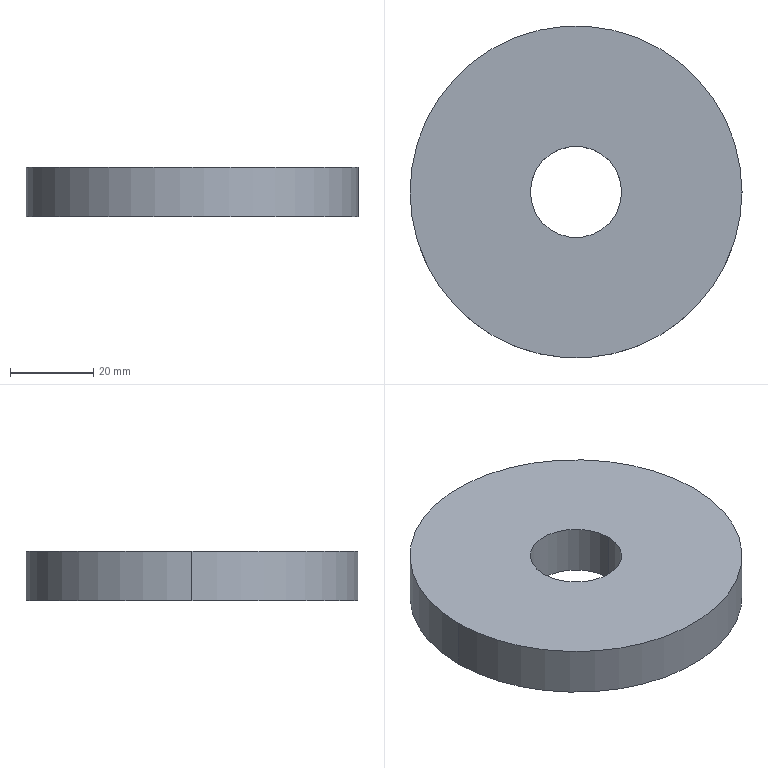Part | SolidWorks | features Extrusion 1 | 1 solid | 6 faces | box 80 x 80 x 12 mm | volume 55757 mm3 | cylinder 4 | plane 2 | commonest cylinder face diameters 22 x2 80 x2
STEP:
#1=CARTESIAN_POINT('',(-11.,0.,12.));
#2=VERTEX_POINT('',#1);
#3=CARTESIAN_POINT('',(11.,0.,12.));
#4=VERTEX_POINT('',#3);
#5=CARTESIAN_POINT('',(0.,0.,12.));
#6=DIRECTION('',(0.,0.,1.));
#7=DIRECTION('',(1.,0.,0.));
#8=AXIS2_PLACEMENT_3D('',#5,#6,#7);
#9=CIRCLE('',#8,11.);
#10=EDGE_CURVE('',#2,#4,#9,.T.);
#11=ORIENTED_EDGE('',*,*,#10,.T.);
#12=CARTESIAN_POINT('',(11.,0.,0.));
#13=VERTEX_POINT('',#12);
#14=CARTESIAN_POINT('',(11.,0.,12.));
#15=DIRECTION('',(0.,0.,-1.));
#16=VECTOR('',#15,1000.);
#17=LINE('',#14,#16);
#18=EDGE_CURVE('',#4,#13,#17,.T.);
#19=ORIENTED_EDGE('',*,*,#18,.T.);
#20=CARTESIAN_POINT('',(-11.,0.,0.));
#21=VERTEX_POINT('',#20);
#22=CARTESIAN_POINT('',(0.,0.,0.));
#23=DIRECTION('',(0.,0.,1.));
#24=DIRECTION('',(1.,0.,0.));
#25=AXIS2_PLACEMENT_3D('',#22,#23,#24);
#26=CIRCLE('',#25,11.);
#27=EDGE_CURVE('',#21,#13,#26,.T.);
#28=ORIENTED_EDGE('',*,*,#27,.F.);
#29=CARTESIAN_POINT('',(-11.,0.,12.));
#30=DIRECTION('',(0.,0.,-1.));
#31=VECTOR('',#30,1000.);
#32=LINE('',#29,#31);
#33=EDGE_CURVE('',#2,#21,#32,.T.);
#34=ORIENTED_EDGE('',*,*,#33,.F.);
#35=EDGE_LOOP('',(#11,#19,#28,#34));
#36=FACE_OUTER_BOUND('',#35,.T.);
#37=CARTESIAN_POINT('',(0.,0.,12.));
#38=DIRECTION('',(0.,0.,-1.));
#39=DIRECTION('',(-1.,0.,0.));
#40=AXIS2_PLACEMENT_3D('',#37,#38,#39);
#41=CYLINDRICAL_SURFACE('',#40,11.);
#42=ADVANCED_FACE('',(#36),#41,.F.);
#43=CARTESIAN_POINT('',(40.,0.,12.));
#44=VERTEX_POINT('',#43);
#45=CARTESIAN_POINT('',(-40.,0.,12.));
#46=VERTEX_POINT('',#45);
#47=CARTESIAN_POINT('',(0.,0.,12.));
#48=DIRECTION('',(0.,0.,1.));
#49=DIRECTION('',(1.,0.,0.));
#50=AXIS2_PLACEMENT_3D('',#47,#48,#49);
#51=CIRCLE('',#50,40.);
#52=EDGE_CURVE('',#44,#46,#51,.T.);
#53=ORIENTED_EDGE('',*,*,#52,.F.);
#54=CARTESIAN_POINT('',(40.,0.,0.));
#55=VERTEX_POINT('',#54);
#56=CARTESIAN_POINT('',(40.,0.,12.));
#57=DIRECTION('',(0.,0.,-1.));
#58=VECTOR('',#57,1000.);
#59=LINE('',#56,#58);
#60=EDGE_CURVE('',#44,#55,#59,.T.);
#61=ORIENTED_EDGE('',*,*,#60,.T.);
#62=CARTESIAN_POINT('',(-40.,0.,0.));
#63=VERTEX_POINT('',#62);
#64=CARTESIAN_POINT('',(0.,0.,0.));
#65=DIRECTION('',(0.,0.,1.));
#66=DIRECTION('',(1.,0.,0.));
#67=AXIS2_PLACEMENT_3D('',#64,#65,#66);
#68=CIRCLE('',#67,40.);
#69=EDGE_CURVE('',#55,#63,#68,.T.);
#70=ORIENTED_EDGE('',*,*,#69,.T.);
#71=CARTESIAN_POINT('',(-40.,0.,12.));
#72=DIRECTION('',(0.,0.,-1.));
#73=VECTOR('',#72,1000.);
#74=LINE('',#71,#73);
#75=EDGE_CURVE('',#46,#63,#74,.T.);
#76=ORIENTED_EDGE('',*,*,#75,.F.);
#77=EDGE_LOOP('',(#53,#61,#70,#76));
#78=FACE_OUTER_BOUND('',#77,.T.);
#79=CARTESIAN_POINT('',(0.,0.,12.));
#80=DIRECTION('',(0.,0.,-1.));
#81=DIRECTION('',(-1.,0.,0.));
#82=AXIS2_PLACEMENT_3D('',#79,#80,#81);
#83=CYLINDRICAL_SURFACE('',#82,40.);
#84=ADVANCED_FACE('',(#78),#83,.T.);
#85=CARTESIAN_POINT('',(0.,0.,12.));
#86=DIRECTION('',(0.,0.,1.));
#87=DIRECTION('',(1.,0.,0.));
#88=AXIS2_PLACEMENT_3D('',#85,#86,#87);
#89=CIRCLE('',#88,40.);
#90=EDGE_CURVE('',#46,#44,#89,.T.);
#91=ORIENTED_EDGE('',*,*,#90,.T.);
#92=ORIENTED_EDGE('',*,*,#52,.T.);
#93=EDGE_LOOP('',(#91,#92));
#94=FACE_OUTER_BOUND('',#93,.T.);
#95=ORIENTED_EDGE('',*,*,#10,.F.);
#96=CARTESIAN_POINT('',(0.,0.,12.));
#97=DIRECTION('',(0.,0.,1.));
#98=DIRECTION('',(1.,0.,0.));
#99=AXIS2_PLACEMENT_3D('',#96,#97,#98);
#100=CIRCLE('',#99,11.);
#101=EDGE_CURVE('',#4,#2,#100,.T.);
#102=ORIENTED_EDGE('',*,*,#101,.F.);
#103=EDGE_LOOP('',(#95,#102));
#104=FACE_BOUND('',#103,.T.);
#105=CARTESIAN_POINT('',(0.,0.,12.));
#106=DIRECTION('',(0.,0.,1.));
#107=DIRECTION('',(1.,0.,0.));
#108=AXIS2_PLACEMENT_3D('',#105,#106,#107);
#109=PLANE('',#108);
#110=ADVANCED_FACE('',(#94,#104),#109,.T.);
#111=CARTESIAN_POINT('',(0.,0.,0.));
#112=DIRECTION('',(0.,0.,1.));
#113=DIRECTION('',(1.,0.,0.));
#114=AXIS2_PLACEMENT_3D('',#111,#112,#113);
#115=CIRCLE('',#114,40.);
#116=EDGE_CURVE('',#63,#55,#115,.T.);
#117=ORIENTED_EDGE('',*,*,#116,.F.);
#118=ORIENTED_EDGE('',*,*,#69,.F.);
#119=EDGE_LOOP('',(#117,#118));
#120=FACE_OUTER_BOUND('',#119,.T.);
#121=ORIENTED_EDGE('',*,*,#27,.T.);
#122=CARTESIAN_POINT('',(0.,0.,0.));
#123=DIRECTION('',(0.,0.,1.));
#124=DIRECTION('',(1.,0.,0.));
#125=AXIS2_PLACEMENT_3D('',#122,#123,#124);
#126=CIRCLE('',#125,11.);
#127=EDGE_CURVE('',#13,#21,#126,.T.);
#128=ORIENTED_EDGE('',*,*,#127,.T.);
#129=EDGE_LOOP('',(#121,#128));
#130=FACE_BOUND('',#129,.T.);
#131=CARTESIAN_POINT('',(0.,0.,0.));
#132=DIRECTION('',(0.,0.,1.));
#133=DIRECTION('',(1.,0.,0.));
#134=AXIS2_PLACEMENT_3D('',#131,#132,#133);
#135=PLANE('',#134);
#136=ADVANCED_FACE('',(#120,#130),#135,.F.);
#137=ORIENTED_EDGE('',*,*,#60,.F.);
#138=ORIENTED_EDGE('',*,*,#90,.F.);
#139=ORIENTED_EDGE('',*,*,#75,.T.);
#140=ORIENTED_EDGE('',*,*,#116,.T.);
#141=EDGE_LOOP('',(#137,#138,#139,#140));
#142=FACE_OUTER_BOUND('',#141,.T.);
#143=CARTESIAN_POINT('',(0.,0.,12.));
#144=DIRECTION('',(0.,0.,-1.));
#145=DIRECTION('',(-1.,0.,0.));
#146=AXIS2_PLACEMENT_3D('',#143,#144,#145);
#147=CYLINDRICAL_SURFACE('',#146,40.);
#148=ADVANCED_FACE('',(#142),#147,.T.);
#149=ORIENTED_EDGE('',*,*,#18,.F.);
#150=ORIENTED_EDGE('',*,*,#101,.T.);
#151=ORIENTED_EDGE('',*,*,#33,.T.);
#152=ORIENTED_EDGE('',*,*,#127,.F.);
#153=EDGE_LOOP('',(#149,#150,#151,#152));
#154=FACE_OUTER_BOUND('',#153,.T.);
#155=CARTESIAN_POINT('',(0.,0.,12.));
#156=DIRECTION('',(0.,0.,-1.));
#157=DIRECTION('',(-1.,0.,0.));
#158=AXIS2_PLACEMENT_3D('',#155,#156,#157);
#159=CYLINDRICAL_SURFACE('',#158,11.);
#160=ADVANCED_FACE('',(#154),#159,.F.);
#161=CLOSED_SHELL('',(#42,#84,#110,#136,#148,#160));
#162=MANIFOLD_SOLID_BREP('',#161);
#163=CARTESIAN_POINT('',(0.,0.,0.));
#164=DIRECTION('',(0.,0.,1.));
#165=DIRECTION('',(1.,0.,0.));
#166=AXIS2_PLACEMENT_3D('',#163,#164,#165);
#167=(LENGTH_UNIT()NAMED_UNIT(*)SI_UNIT(.MILLI.,.METRE.));
#168=UNCERTAINTY_MEASURE_WITH_UNIT(LENGTH_MEASURE(0.00001),#167,'','');
#169=(NAMED_UNIT(*)PLANE_ANGLE_UNIT()SI_UNIT($,.RADIAN.));
#170=(NAMED_UNIT(*)SI_UNIT($,.STERADIAN.)SOLID_ANGLE_UNIT());
#171=(GEOMETRIC_REPRESENTATION_CONTEXT(3)GLOBAL_UNCERTAINTY_ASSIGNED_CONTEXT((#168))GLOBAL_UNIT_ASSIGNED_CONTEXT((#167,#169,#170))REPRESENTATION_CONTEXT('',''));
#172=ADVANCED_BREP_SHAPE_REPRESENTATION('',(#162,#166),#171);